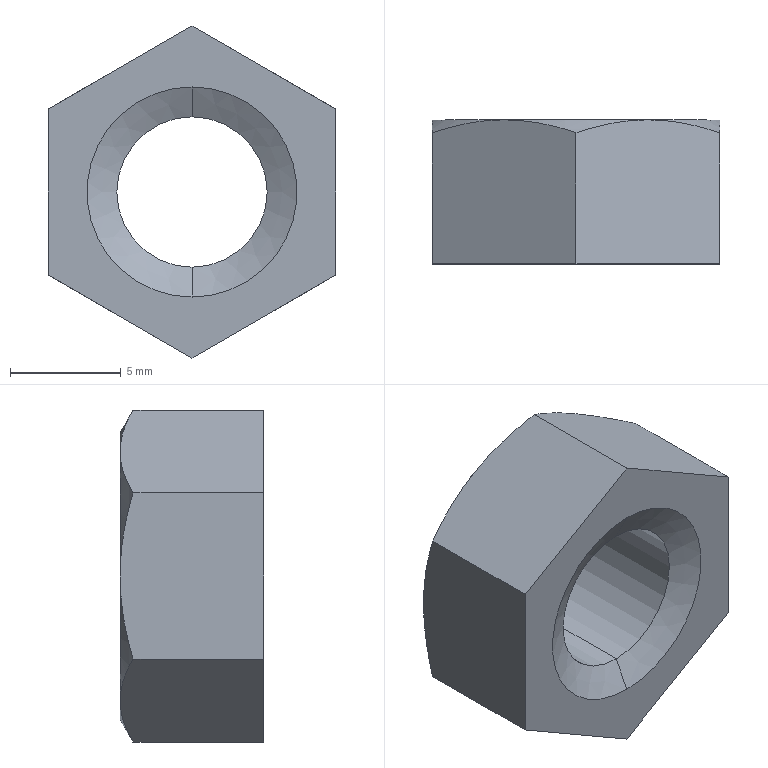Part | STEP file | 0244_308_SLBNR8 | 1 solid | 21 faces | box 13 x 6.5 x 15.011 mm | volume 690.678 mm3 | cone 11 | plane 8 | cylinder 2 | commonest cylinder face diameters 6.8 x2